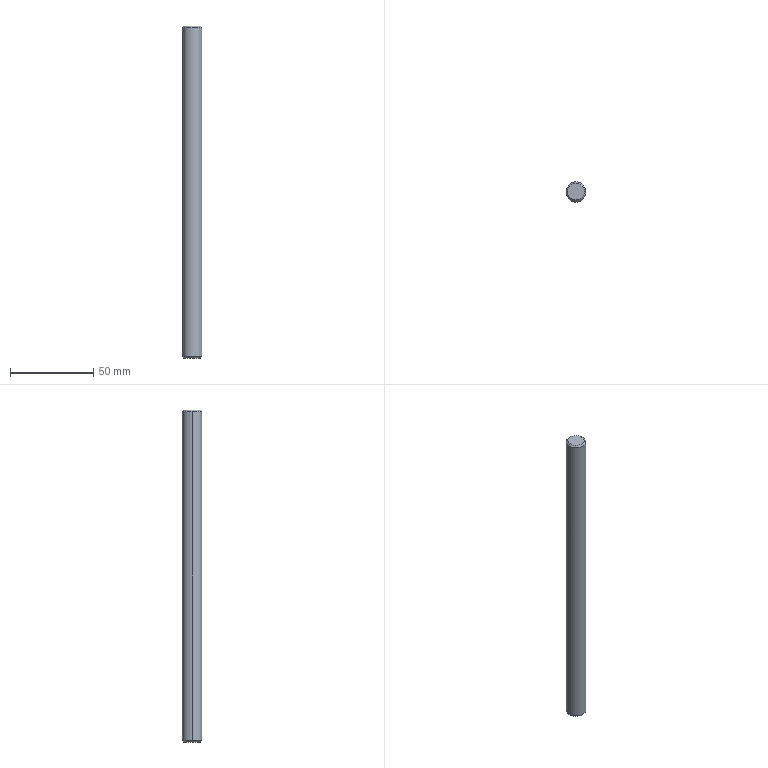Part | STEP file | X77-08203 | 1 solid | 8 faces | box 12 x 12 x 200 mm | volume 22584 mm3 | cone 4 | cylinder 2 | plane 2 | commonest cylinder face diameters 12 x2
STEP:
#1=CARTESIAN_POINT('',(5.,2660.092,200.));
#2=VERTEX_POINT('',#1);
#3=CARTESIAN_POINT('',(-5.,2660.092,200.));
#4=VERTEX_POINT('',#3);
#5=CARTESIAN_POINT('',(0.000000001,2660.092,200.));
#6=DIRECTION('',(0.,0.,1.));
#7=DIRECTION('',(1.,0.,0.));
#8=AXIS2_PLACEMENT_3D('',#5,#6,#7);
#9=CIRCLE('',#8,5.);
#10=EDGE_CURVE('',#2,#4,#9,.T.);
#11=ORIENTED_EDGE('',*,*,#10,.F.);
#12=CARTESIAN_POINT('',(6.,2660.092,199.));
#13=VERTEX_POINT('',#12);
#14=CARTESIAN_POINT('',(5.,2660.092,200.));
#15=DIRECTION('',(0.7071,0.,-0.7071));
#16=VECTOR('',#15,1000.);
#17=LINE('',#14,#16);
#18=EDGE_CURVE('',#2,#13,#17,.T.);
#19=ORIENTED_EDGE('',*,*,#18,.T.);
#20=CARTESIAN_POINT('',(-6.,2660.092,199.));
#21=VERTEX_POINT('',#20);
#22=CARTESIAN_POINT('',(0.000000001,2660.092,199.));
#23=DIRECTION('',(0.,0.,-1.));
#24=DIRECTION('',(1.,0.,0.));
#25=AXIS2_PLACEMENT_3D('',#22,#23,#24);
#26=CIRCLE('',#25,6.);
#27=EDGE_CURVE('',#21,#13,#26,.T.);
#28=ORIENTED_EDGE('',*,*,#27,.F.);
#29=CARTESIAN_POINT('',(-5.,2660.092,200.));
#30=DIRECTION('',(-0.7071,0.,-0.7071));
#31=VECTOR('',#30,1000.);
#32=LINE('',#29,#31);
#33=EDGE_CURVE('',#4,#21,#32,.T.);
#34=ORIENTED_EDGE('',*,*,#33,.F.);
#35=EDGE_LOOP('',(#11,#19,#28,#34));
#36=FACE_OUTER_BOUND('',#35,.T.);
#37=CARTESIAN_POINT('',(0.000000001,2660.092,200.));
#38=DIRECTION('',(0.,0.,-1.));
#39=DIRECTION('',(-1.,0.,0.));
#40=AXIS2_PLACEMENT_3D('',#37,#38,#39);
#41=CONICAL_SURFACE('',#40,5.,0.7854);
#42=ADVANCED_FACE('',(#36),#41,.T.);
#43=CARTESIAN_POINT('',(-5.,2660.092,0.));
#44=VERTEX_POINT('',#43);
#45=CARTESIAN_POINT('',(5.,2660.092,0.));
#46=VERTEX_POINT('',#45);
#47=CARTESIAN_POINT('',(0.000000001,2660.092,0.));
#48=DIRECTION('',(0.,0.,-1.));
#49=DIRECTION('',(1.,0.,0.));
#50=AXIS2_PLACEMENT_3D('',#47,#48,#49);
#51=CIRCLE('',#50,5.);
#52=EDGE_CURVE('',#44,#46,#51,.T.);
#53=ORIENTED_EDGE('',*,*,#52,.F.);
#54=CARTESIAN_POINT('',(-6.,2660.092,1.));
#55=VERTEX_POINT('',#54);
#56=CARTESIAN_POINT('',(-6.,2660.092,1.));
#57=DIRECTION('',(-0.7071,0.,0.7071));
#58=VECTOR('',#57,1000.);
#59=LINE('',#56,#58);
#60=EDGE_CURVE('',#44,#55,#59,.T.);
#61=ORIENTED_EDGE('',*,*,#60,.T.);
#62=CARTESIAN_POINT('',(6.,2660.092,1.));
#63=VERTEX_POINT('',#62);
#64=CARTESIAN_POINT('',(0.000000001,2660.092,1.));
#65=DIRECTION('',(0.,0.,1.));
#66=DIRECTION('',(1.,0.,0.));
#67=AXIS2_PLACEMENT_3D('',#64,#65,#66);
#68=CIRCLE('',#67,6.);
#69=EDGE_CURVE('',#63,#55,#68,.T.);
#70=ORIENTED_EDGE('',*,*,#69,.F.);
#71=CARTESIAN_POINT('',(6.,2660.092,1.));
#72=DIRECTION('',(0.7071,0.,0.7071));
#73=VECTOR('',#72,1000.);
#74=LINE('',#71,#73);
#75=EDGE_CURVE('',#46,#63,#74,.T.);
#76=ORIENTED_EDGE('',*,*,#75,.F.);
#77=EDGE_LOOP('',(#53,#61,#70,#76));
#78=FACE_OUTER_BOUND('',#77,.T.);
#79=CARTESIAN_POINT('',(0.000000001,2660.092,1.));
#80=DIRECTION('',(0.,0.,1.));
#81=DIRECTION('',(1.,0.,0.));
#82=AXIS2_PLACEMENT_3D('',#79,#80,#81);
#83=CONICAL_SURFACE('',#82,6.,0.7854);
#84=ADVANCED_FACE('',(#78),#83,.T.);
#85=ORIENTED_EDGE('',*,*,#27,.T.);
#86=CARTESIAN_POINT('',(6.,2660.092,200.));
#87=DIRECTION('',(0.,0.,-1.));
#88=VECTOR('',#87,1000.);
#89=LINE('',#86,#88);
#90=EDGE_CURVE('',#13,#63,#89,.T.);
#91=ORIENTED_EDGE('',*,*,#90,.T.);
#92=ORIENTED_EDGE('',*,*,#69,.T.);
#93=CARTESIAN_POINT('',(-6.,2660.092,200.));
#94=DIRECTION('',(0.,0.,-1.));
#95=VECTOR('',#94,1000.);
#96=LINE('',#93,#95);
#97=EDGE_CURVE('',#21,#55,#96,.T.);
#98=ORIENTED_EDGE('',*,*,#97,.F.);
#99=EDGE_LOOP('',(#85,#91,#92,#98));
#100=FACE_OUTER_BOUND('',#99,.T.);
#101=CARTESIAN_POINT('',(0.000000001,2660.092,200.));
#102=DIRECTION('',(0.,0.,-1.));
#103=DIRECTION('',(-1.,0.,0.));
#104=AXIS2_PLACEMENT_3D('',#101,#102,#103);
#105=CYLINDRICAL_SURFACE('',#104,6.);
#106=ADVANCED_FACE('',(#100),#105,.T.);
#107=ORIENTED_EDGE('',*,*,#90,.F.);
#108=CARTESIAN_POINT('',(0.000000001,2660.092,199.));
#109=DIRECTION('',(0.,0.,-1.));
#110=DIRECTION('',(1.,0.,0.));
#111=AXIS2_PLACEMENT_3D('',#108,#109,#110);
#112=CIRCLE('',#111,6.);
#113=EDGE_CURVE('',#13,#21,#112,.T.);
#114=ORIENTED_EDGE('',*,*,#113,.T.);
#115=ORIENTED_EDGE('',*,*,#97,.T.);
#116=CARTESIAN_POINT('',(0.000000001,2660.092,1.));
#117=DIRECTION('',(0.,0.,1.));
#118=DIRECTION('',(1.,0.,0.));
#119=AXIS2_PLACEMENT_3D('',#116,#117,#118);
#120=CIRCLE('',#119,6.);
#121=EDGE_CURVE('',#55,#63,#120,.T.);
#122=ORIENTED_EDGE('',*,*,#121,.T.);
#123=EDGE_LOOP('',(#107,#114,#115,#122));
#124=FACE_OUTER_BOUND('',#123,.T.);
#125=CARTESIAN_POINT('',(0.000000001,2660.092,200.));
#126=DIRECTION('',(0.,0.,-1.));
#127=DIRECTION('',(-1.,0.,0.));
#128=AXIS2_PLACEMENT_3D('',#125,#126,#127);
#129=CYLINDRICAL_SURFACE('',#128,6.);
#130=ADVANCED_FACE('',(#124),#129,.T.);
#131=CARTESIAN_POINT('',(0.000000001,2660.092,200.));
#132=DIRECTION('',(0.,0.,1.));
#133=DIRECTION('',(1.,0.,0.));
#134=AXIS2_PLACEMENT_3D('',#131,#132,#133);
#135=CIRCLE('',#134,5.);
#136=EDGE_CURVE('',#4,#2,#135,.T.);
#137=ORIENTED_EDGE('',*,*,#136,.T.);
#138=ORIENTED_EDGE('',*,*,#10,.T.);
#139=EDGE_LOOP('',(#137,#138));
#140=FACE_OUTER_BOUND('',#139,.T.);
#141=CARTESIAN_POINT('',(0.000000001,2660.092,200.));
#142=DIRECTION('',(0.,0.,1.));
#143=DIRECTION('',(1.,0.,0.));
#144=AXIS2_PLACEMENT_3D('',#141,#142,#143);
#145=PLANE('',#144);
#146=ADVANCED_FACE('',(#140),#145,.T.);
#147=CARTESIAN_POINT('',(0.000000001,2660.092,0.));
#148=DIRECTION('',(0.,0.,-1.));
#149=DIRECTION('',(1.,0.,0.));
#150=AXIS2_PLACEMENT_3D('',#147,#148,#149);
#151=CIRCLE('',#150,5.);
#152=EDGE_CURVE('',#46,#44,#151,.T.);
#153=ORIENTED_EDGE('',*,*,#152,.T.);
#154=ORIENTED_EDGE('',*,*,#52,.T.);
#155=EDGE_LOOP('',(#153,#154));
#156=FACE_OUTER_BOUND('',#155,.T.);
#157=CARTESIAN_POINT('',(0.000000001,2660.092,0.));
#158=DIRECTION('',(0.,0.,1.));
#159=DIRECTION('',(1.,0.,0.));
#160=AXIS2_PLACEMENT_3D('',#157,#158,#159);
#161=PLANE('',#160);
#162=ADVANCED_FACE('',(#156),#161,.F.);
#163=ORIENTED_EDGE('',*,*,#60,.F.);
#164=ORIENTED_EDGE('',*,*,#152,.F.);
#165=ORIENTED_EDGE('',*,*,#75,.T.);
#166=ORIENTED_EDGE('',*,*,#121,.F.);
#167=EDGE_LOOP('',(#163,#164,#165,#166));
#168=FACE_OUTER_BOUND('',#167,.T.);
#169=CARTESIAN_POINT('',(0.000000001,2660.092,1.));
#170=DIRECTION('',(0.,0.,1.));
#171=DIRECTION('',(1.,0.,0.));
#172=AXIS2_PLACEMENT_3D('',#169,#170,#171);
#173=CONICAL_SURFACE('',#172,6.,0.7854);
#174=ADVANCED_FACE('',(#168),#173,.T.);
#175=ORIENTED_EDGE('',*,*,#18,.F.);
#176=ORIENTED_EDGE('',*,*,#136,.F.);
#177=ORIENTED_EDGE('',*,*,#33,.T.);
#178=ORIENTED_EDGE('',*,*,#113,.F.);
#179=EDGE_LOOP('',(#175,#176,#177,#178));
#180=FACE_OUTER_BOUND('',#179,.T.);
#181=CARTESIAN_POINT('',(0.000000001,2660.092,200.));
#182=DIRECTION('',(0.,0.,-1.));
#183=DIRECTION('',(-1.,0.,0.));
#184=AXIS2_PLACEMENT_3D('',#181,#182,#183);
#185=CONICAL_SURFACE('',#184,5.,0.7854);
#186=ADVANCED_FACE('',(#180),#185,.T.);
#187=CLOSED_SHELL('',(#42,#84,#106,#130,#146,#162,#174,#186));
#188=MANIFOLD_SOLID_BREP('',#187);
#189=CARTESIAN_POINT('',(0.,0.,0.));
#190=DIRECTION('',(0.,0.,1.));
#191=DIRECTION('',(1.,0.,0.));
#192=AXIS2_PLACEMENT_3D('',#189,#190,#191);
#193=(LENGTH_UNIT()NAMED_UNIT(*)SI_UNIT(.MILLI.,.METRE.));
#194=UNCERTAINTY_MEASURE_WITH_UNIT(LENGTH_MEASURE(0.00001),#193,'','');
#195=(NAMED_UNIT(*)PLANE_ANGLE_UNIT()SI_UNIT($,.RADIAN.));
#196=(NAMED_UNIT(*)SI_UNIT($,.STERADIAN.)SOLID_ANGLE_UNIT());
#197=(GEOMETRIC_REPRESENTATION_CONTEXT(3)GLOBAL_UNCERTAINTY_ASSIGNED_CONTEXT((#194))GLOBAL_UNIT_ASSIGNED_CONTEXT((#193,#195,#196))REPRESENTATION_CONTEXT('',''));
#198=ADVANCED_BREP_SHAPE_REPRESENTATION('',(#188,#192),#197);